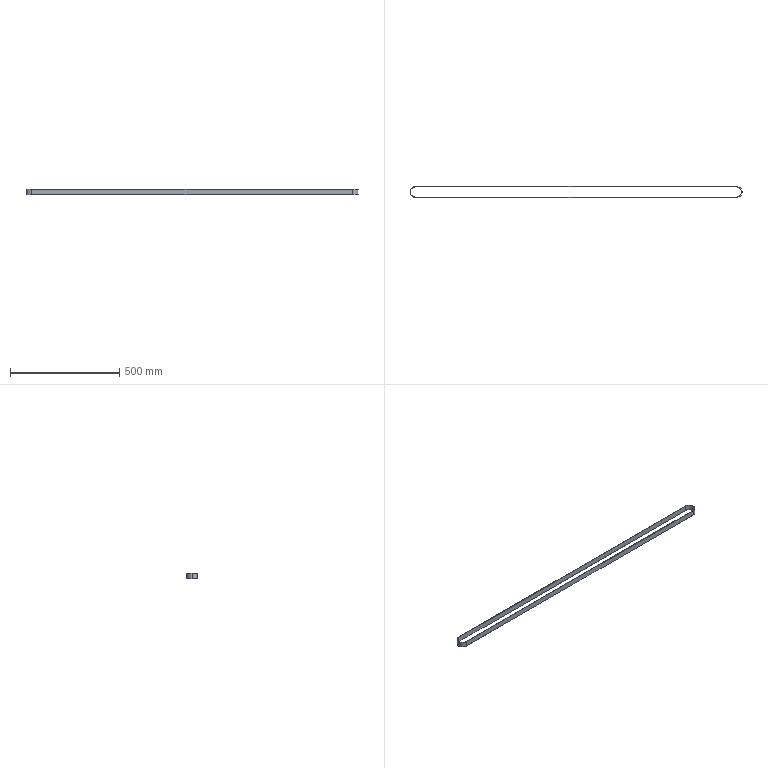Part | SolidWorks | features BaseBody 1 | 1 solid | 12 faces | box 1519 x 50.79 x 25 mm | volume 154464 mm3 | plane 6 | cylinder 6 | commonest cylinder face diameters 46.79 x3 50.79 x3
STEP:
#1=CARTESIAN_POINT('',(1368.,13.395,-12.5));
#2=VERTEX_POINT('',#1);
#3=CARTESIAN_POINT('',(-100.,13.395,-12.5));
#4=VERTEX_POINT('',#3);
#5=CARTESIAN_POINT('',(-100.,13.395,-12.5));
#6=DIRECTION('',(-1.,0.,0.));
#7=VECTOR('',#6,1000.);
#8=LINE('',#5,#7);
#9=EDGE_CURVE('',#2,#4,#8,.T.);
#10=ORIENTED_EDGE('',*,*,#9,.F.);
#11=CARTESIAN_POINT('',(1368.,13.395,12.5));
#12=VERTEX_POINT('',#11);
#13=CARTESIAN_POINT('',(1368.,13.395,12.5));
#14=DIRECTION('',(0.,0.,-1.));
#15=VECTOR('',#14,1000.);
#16=LINE('',#13,#15);
#17=EDGE_CURVE('',#12,#2,#16,.T.);
#18=ORIENTED_EDGE('',*,*,#17,.F.);
#19=CARTESIAN_POINT('',(-100.,13.395,12.5));
#20=VERTEX_POINT('',#19);
#21=CARTESIAN_POINT('',(-100.,13.395,12.5));
#22=DIRECTION('',(-1.,0.,0.));
#23=VECTOR('',#22,1000.);
#24=LINE('',#21,#23);
#25=EDGE_CURVE('',#12,#20,#24,.T.);
#26=ORIENTED_EDGE('',*,*,#25,.T.);
#27=CARTESIAN_POINT('',(-100.,13.395,12.5));
#28=DIRECTION('',(0.,0.,-1.));
#29=VECTOR('',#28,1000.);
#30=LINE('',#27,#29);
#31=EDGE_CURVE('',#20,#4,#30,.T.);
#32=ORIENTED_EDGE('',*,*,#31,.T.);
#33=EDGE_LOOP('',(#10,#18,#26,#32));
#34=FACE_OUTER_BOUND('',#33,.T.);
#35=CARTESIAN_POINT('',(-100.,13.395,12.5));
#36=DIRECTION('',(0.,-1.,0.));
#37=DIRECTION('',(0.,0.,-1.));
#38=AXIS2_PLACEMENT_3D('',#35,#36,#37);
#39=PLANE('',#38);
#40=ADVANCED_FACE('',(#34),#39,.T.);
#41=CARTESIAN_POINT('',(1368.,-33.395,-12.5));
#42=VERTEX_POINT('',#41);
#43=CARTESIAN_POINT('',(1368.,-10.,-12.5));
#44=DIRECTION('',(0.,0.,1.));
#45=DIRECTION('',(-1.,0.,0.));
#46=AXIS2_PLACEMENT_3D('',#43,#44,#45);
#47=CIRCLE('',#46,23.395);
#48=EDGE_CURVE('',#42,#2,#47,.T.);
#49=ORIENTED_EDGE('',*,*,#48,.F.);
#50=CARTESIAN_POINT('',(1368.,-33.395,12.5));
#51=VERTEX_POINT('',#50);
#52=CARTESIAN_POINT('',(1368.,-33.395,12.5));
#53=DIRECTION('',(0.,0.,-1.));
#54=VECTOR('',#53,1000.);
#55=LINE('',#52,#54);
#56=EDGE_CURVE('',#51,#42,#55,.T.);
#57=ORIENTED_EDGE('',*,*,#56,.F.);
#58=CARTESIAN_POINT('',(1368.,-10.,12.5));
#59=DIRECTION('',(0.,0.,1.));
#60=DIRECTION('',(-1.,0.,0.));
#61=AXIS2_PLACEMENT_3D('',#58,#59,#60);
#62=CIRCLE('',#61,23.395);
#63=EDGE_CURVE('',#51,#12,#62,.T.);
#64=ORIENTED_EDGE('',*,*,#63,.T.);
#65=ORIENTED_EDGE('',*,*,#17,.T.);
#66=EDGE_LOOP('',(#49,#57,#64,#65));
#67=FACE_OUTER_BOUND('',#66,.T.);
#68=CARTESIAN_POINT('',(1368.,-10.,12.5));
#69=DIRECTION('',(0.,0.,-1.));
#70=DIRECTION('',(-1.,0.,0.));
#71=AXIS2_PLACEMENT_3D('',#68,#69,#70);
#72=CYLINDRICAL_SURFACE('',#71,23.395);
#73=ADVANCED_FACE('',(#67),#72,.F.);
#74=CARTESIAN_POINT('',(-100.,-33.395,-12.5));
#75=VERTEX_POINT('',#74);
#76=CARTESIAN_POINT('',(1368.,-33.395,-12.5));
#77=DIRECTION('',(1.,0.,0.));
#78=VECTOR('',#77,1000.);
#79=LINE('',#76,#78);
#80=EDGE_CURVE('',#75,#42,#79,.T.);
#81=ORIENTED_EDGE('',*,*,#80,.F.);
#82=CARTESIAN_POINT('',(-100.,-33.395,12.5));
#83=VERTEX_POINT('',#82);
#84=CARTESIAN_POINT('',(-100.,-33.395,12.5));
#85=DIRECTION('',(0.,0.,-1.));
#86=VECTOR('',#85,1000.);
#87=LINE('',#84,#86);
#88=EDGE_CURVE('',#83,#75,#87,.T.);
#89=ORIENTED_EDGE('',*,*,#88,.F.);
#90=CARTESIAN_POINT('',(1368.,-33.395,12.5));
#91=DIRECTION('',(1.,0.,0.));
#92=VECTOR('',#91,1000.);
#93=LINE('',#90,#92);
#94=EDGE_CURVE('',#83,#51,#93,.T.);
#95=ORIENTED_EDGE('',*,*,#94,.T.);
#96=ORIENTED_EDGE('',*,*,#56,.T.);
#97=EDGE_LOOP('',(#81,#89,#95,#96));
#98=FACE_OUTER_BOUND('',#97,.T.);
#99=CARTESIAN_POINT('',(1368.,-33.395,12.5));
#100=DIRECTION('',(0.,1.,0.));
#101=DIRECTION('',(1.,0.,0.));
#102=AXIS2_PLACEMENT_3D('',#99,#100,#101);
#103=PLANE('',#102);
#104=ADVANCED_FACE('',(#98),#103,.T.);
#105=CARTESIAN_POINT('',(-123.395,-10.,12.5));
#106=VERTEX_POINT('',#105);
#107=CARTESIAN_POINT('',(-123.395,-10.,-12.5));
#108=VERTEX_POINT('',#107);
#109=CARTESIAN_POINT('',(-123.395,-10.,12.5));
#110=DIRECTION('',(0.,0.,-1.));
#111=VECTOR('',#110,1000.);
#112=LINE('',#109,#111);
#113=EDGE_CURVE('',#106,#108,#112,.T.);
#114=ORIENTED_EDGE('',*,*,#113,.F.);
#115=CARTESIAN_POINT('',(-100.,-10.,12.5));
#116=DIRECTION('',(0.,0.,1.));
#117=DIRECTION('',(-1.,0.,0.));
#118=AXIS2_PLACEMENT_3D('',#115,#116,#117);
#119=CIRCLE('',#118,23.395);
#120=EDGE_CURVE('',#106,#83,#119,.T.);
#121=ORIENTED_EDGE('',*,*,#120,.T.);
#122=ORIENTED_EDGE('',*,*,#88,.T.);
#123=CARTESIAN_POINT('',(-100.,-10.,-12.5));
#124=DIRECTION('',(0.,0.,1.));
#125=DIRECTION('',(-1.,0.,0.));
#126=AXIS2_PLACEMENT_3D('',#123,#124,#125);
#127=CIRCLE('',#126,23.395);
#128=EDGE_CURVE('',#108,#75,#127,.T.);
#129=ORIENTED_EDGE('',*,*,#128,.F.);
#130=EDGE_LOOP('',(#114,#121,#122,#129));
#131=FACE_OUTER_BOUND('',#130,.T.);
#132=CARTESIAN_POINT('',(-100.,-10.,12.5));
#133=DIRECTION('',(0.,0.,-1.));
#134=DIRECTION('',(-1.,0.,0.));
#135=AXIS2_PLACEMENT_3D('',#132,#133,#134);
#136=CYLINDRICAL_SURFACE('',#135,23.395);
#137=ADVANCED_FACE('',(#131),#136,.F.);
#138=CARTESIAN_POINT('',(1368.,15.395,-12.5));
#139=VERTEX_POINT('',#138);
#140=CARTESIAN_POINT('',(-100.,15.395,-12.5));
#141=VERTEX_POINT('',#140);
#142=CARTESIAN_POINT('',(-100.,15.395,-12.5));
#143=DIRECTION('',(-1.,0.,0.));
#144=VECTOR('',#143,1000.);
#145=LINE('',#142,#144);
#146=EDGE_CURVE('',#139,#141,#145,.T.);
#147=ORIENTED_EDGE('',*,*,#146,.T.);
#148=CARTESIAN_POINT('',(-100.,15.395,12.5));
#149=VERTEX_POINT('',#148);
#150=CARTESIAN_POINT('',(-100.,15.395,12.5));
#151=DIRECTION('',(0.,0.,-1.));
#152=VECTOR('',#151,1000.);
#153=LINE('',#150,#152);
#154=EDGE_CURVE('',#149,#141,#153,.T.);
#155=ORIENTED_EDGE('',*,*,#154,.F.);
#156=CARTESIAN_POINT('',(1368.,15.395,12.5));
#157=VERTEX_POINT('',#156);
#158=CARTESIAN_POINT('',(-100.,15.395,12.5));
#159=DIRECTION('',(-1.,0.,0.));
#160=VECTOR('',#159,1000.);
#161=LINE('',#158,#160);
#162=EDGE_CURVE('',#157,#149,#161,.T.);
#163=ORIENTED_EDGE('',*,*,#162,.F.);
#164=CARTESIAN_POINT('',(1368.,15.395,12.5));
#165=DIRECTION('',(0.,0.,-1.));
#166=VECTOR('',#165,1000.);
#167=LINE('',#164,#166);
#168=EDGE_CURVE('',#157,#139,#167,.T.);
#169=ORIENTED_EDGE('',*,*,#168,.T.);
#170=EDGE_LOOP('',(#147,#155,#163,#169));
#171=FACE_OUTER_BOUND('',#170,.T.);
#172=CARTESIAN_POINT('',(-100.,15.395,12.5));
#173=DIRECTION('',(0.,-1.,0.));
#174=DIRECTION('',(0.,0.,-1.));
#175=AXIS2_PLACEMENT_3D('',#172,#173,#174);
#176=PLANE('',#175);
#177=ADVANCED_FACE('',(#171),#176,.F.);
#178=CARTESIAN_POINT('',(1368.,-35.395,-12.5));
#179=VERTEX_POINT('',#178);
#180=CARTESIAN_POINT('',(1368.,-10.,-12.5));
#181=DIRECTION('',(0.,0.,1.));
#182=DIRECTION('',(-1.,0.,0.));
#183=AXIS2_PLACEMENT_3D('',#180,#181,#182);
#184=CIRCLE('',#183,25.395);
#185=EDGE_CURVE('',#179,#139,#184,.T.);
#186=ORIENTED_EDGE('',*,*,#185,.T.);
#187=ORIENTED_EDGE('',*,*,#168,.F.);
#188=CARTESIAN_POINT('',(1368.,-35.395,12.5));
#189=VERTEX_POINT('',#188);
#190=CARTESIAN_POINT('',(1368.,-10.,12.5));
#191=DIRECTION('',(0.,0.,1.));
#192=DIRECTION('',(-1.,0.,0.));
#193=AXIS2_PLACEMENT_3D('',#190,#191,#192);
#194=CIRCLE('',#193,25.395);
#195=EDGE_CURVE('',#189,#157,#194,.T.);
#196=ORIENTED_EDGE('',*,*,#195,.F.);
#197=CARTESIAN_POINT('',(1368.,-35.395,12.5));
#198=DIRECTION('',(0.,0.,-1.));
#199=VECTOR('',#198,1000.);
#200=LINE('',#197,#199);
#201=EDGE_CURVE('',#189,#179,#200,.T.);
#202=ORIENTED_EDGE('',*,*,#201,.T.);
#203=EDGE_LOOP('',(#186,#187,#196,#202));
#204=FACE_OUTER_BOUND('',#203,.T.);
#205=CARTESIAN_POINT('',(1368.,-10.,12.5));
#206=DIRECTION('',(0.,0.,-1.));
#207=DIRECTION('',(-1.,0.,0.));
#208=AXIS2_PLACEMENT_3D('',#205,#206,#207);
#209=CYLINDRICAL_SURFACE('',#208,25.395);
#210=ADVANCED_FACE('',(#204),#209,.T.);
#211=CARTESIAN_POINT('',(-100.,-35.395,-12.5));
#212=VERTEX_POINT('',#211);
#213=CARTESIAN_POINT('',(-100.,-35.395,-12.5));
#214=DIRECTION('',(1.,0.,0.));
#215=VECTOR('',#214,1000.);
#216=LINE('',#213,#215);
#217=EDGE_CURVE('',#212,#179,#216,.T.);
#218=ORIENTED_EDGE('',*,*,#217,.T.);
#219=ORIENTED_EDGE('',*,*,#201,.F.);
#220=CARTESIAN_POINT('',(-100.,-35.395,12.5));
#221=VERTEX_POINT('',#220);
#222=CARTESIAN_POINT('',(-100.,-35.395,12.5));
#223=DIRECTION('',(1.,0.,0.));
#224=VECTOR('',#223,1000.);
#225=LINE('',#222,#224);
#226=EDGE_CURVE('',#221,#189,#225,.T.);
#227=ORIENTED_EDGE('',*,*,#226,.F.);
#228=CARTESIAN_POINT('',(-100.,-35.395,12.5));
#229=DIRECTION('',(0.,0.,-1.));
#230=VECTOR('',#229,1000.);
#231=LINE('',#228,#230);
#232=EDGE_CURVE('',#221,#212,#231,.T.);
#233=ORIENTED_EDGE('',*,*,#232,.T.);
#234=EDGE_LOOP('',(#218,#219,#227,#233));
#235=FACE_OUTER_BOUND('',#234,.T.);
#236=CARTESIAN_POINT('',(-100.,-35.395,12.5));
#237=DIRECTION('',(0.,1.,0.));
#238=DIRECTION('',(1.,0.,0.));
#239=AXIS2_PLACEMENT_3D('',#236,#237,#238);
#240=PLANE('',#239);
#241=ADVANCED_FACE('',(#235),#240,.F.);
#242=CARTESIAN_POINT('',(-125.395,-10.,12.5));
#243=VERTEX_POINT('',#242);
#244=CARTESIAN_POINT('',(-125.395,-10.,-12.5));
#245=VERTEX_POINT('',#244);
#246=CARTESIAN_POINT('',(-125.395,-10.,12.5));
#247=DIRECTION('',(0.,0.,-1.));
#248=VECTOR('',#247,1000.);
#249=LINE('',#246,#248);
#250=EDGE_CURVE('',#243,#245,#249,.T.);
#251=ORIENTED_EDGE('',*,*,#250,.F.);
#252=CARTESIAN_POINT('',(-100.,-10.,12.5));
#253=DIRECTION('',(0.,0.,1.));
#254=DIRECTION('',(-1.,0.,0.));
#255=AXIS2_PLACEMENT_3D('',#252,#253,#254);
#256=CIRCLE('',#255,25.395);
#257=EDGE_CURVE('',#149,#243,#256,.T.);
#258=ORIENTED_EDGE('',*,*,#257,.F.);
#259=ORIENTED_EDGE('',*,*,#154,.T.);
#260=CARTESIAN_POINT('',(-100.,-10.,-12.5));
#261=DIRECTION('',(0.,0.,1.));
#262=DIRECTION('',(-1.,0.,0.));
#263=AXIS2_PLACEMENT_3D('',#260,#261,#262);
#264=CIRCLE('',#263,25.395);
#265=EDGE_CURVE('',#141,#245,#264,.T.);
#266=ORIENTED_EDGE('',*,*,#265,.T.);
#267=EDGE_LOOP('',(#251,#258,#259,#266));
#268=FACE_OUTER_BOUND('',#267,.T.);
#269=CARTESIAN_POINT('',(-100.,-10.,12.5));
#270=DIRECTION('',(0.,0.,-1.));
#271=DIRECTION('',(-1.,0.,0.));
#272=AXIS2_PLACEMENT_3D('',#269,#270,#271);
#273=CYLINDRICAL_SURFACE('',#272,25.395);
#274=ADVANCED_FACE('',(#268),#273,.T.);
#275=ORIENTED_EDGE('',*,*,#9,.T.);
#276=CARTESIAN_POINT('',(-100.,-10.,-12.5));
#277=DIRECTION('',(0.,0.,1.));
#278=DIRECTION('',(-1.,0.,0.));
#279=AXIS2_PLACEMENT_3D('',#276,#277,#278);
#280=CIRCLE('',#279,23.395);
#281=EDGE_CURVE('',#4,#108,#280,.T.);
#282=ORIENTED_EDGE('',*,*,#281,.T.);
#283=ORIENTED_EDGE('',*,*,#128,.T.);
#284=ORIENTED_EDGE('',*,*,#80,.T.);
#285=ORIENTED_EDGE('',*,*,#48,.T.);
#286=EDGE_LOOP('',(#275,#282,#283,#284,#285));
#287=FACE_BOUND('',#286,.T.);
#288=ORIENTED_EDGE('',*,*,#265,.F.);
#289=ORIENTED_EDGE('',*,*,#146,.F.);
#290=ORIENTED_EDGE('',*,*,#185,.F.);
#291=ORIENTED_EDGE('',*,*,#217,.F.);
#292=CARTESIAN_POINT('',(-100.,-10.,-12.5));
#293=DIRECTION('',(0.,0.,1.));
#294=DIRECTION('',(-1.,0.,0.));
#295=AXIS2_PLACEMENT_3D('',#292,#293,#294);
#296=CIRCLE('',#295,25.395);
#297=EDGE_CURVE('',#245,#212,#296,.T.);
#298=ORIENTED_EDGE('',*,*,#297,.F.);
#299=EDGE_LOOP('',(#288,#289,#290,#291,#298));
#300=FACE_OUTER_BOUND('',#299,.T.);
#301=CARTESIAN_POINT('',(-100.,-10.,-12.5));
#302=DIRECTION('',(0.,0.,-1.));
#303=DIRECTION('',(0.,-1.,0.));
#304=AXIS2_PLACEMENT_3D('',#301,#302,#303);
#305=PLANE('',#304);
#306=ADVANCED_FACE('',(#287,#300),#305,.T.);
#307=CARTESIAN_POINT('',(-100.,-10.,12.5));
#308=DIRECTION('',(0.,0.,1.));
#309=DIRECTION('',(-1.,0.,0.));
#310=AXIS2_PLACEMENT_3D('',#307,#308,#309);
#311=CIRCLE('',#310,23.395);
#312=EDGE_CURVE('',#20,#106,#311,.T.);
#313=ORIENTED_EDGE('',*,*,#312,.F.);
#314=ORIENTED_EDGE('',*,*,#25,.F.);
#315=ORIENTED_EDGE('',*,*,#63,.F.);
#316=ORIENTED_EDGE('',*,*,#94,.F.);
#317=ORIENTED_EDGE('',*,*,#120,.F.);
#318=EDGE_LOOP('',(#313,#314,#315,#316,#317));
#319=FACE_BOUND('',#318,.T.);
#320=ORIENTED_EDGE('',*,*,#257,.T.);
#321=CARTESIAN_POINT('',(-100.,-10.,12.5));
#322=DIRECTION('',(0.,0.,1.));
#323=DIRECTION('',(-1.,0.,0.));
#324=AXIS2_PLACEMENT_3D('',#321,#322,#323);
#325=CIRCLE('',#324,25.395);
#326=EDGE_CURVE('',#243,#221,#325,.T.);
#327=ORIENTED_EDGE('',*,*,#326,.T.);
#328=ORIENTED_EDGE('',*,*,#226,.T.);
#329=ORIENTED_EDGE('',*,*,#195,.T.);
#330=ORIENTED_EDGE('',*,*,#162,.T.);
#331=EDGE_LOOP('',(#320,#327,#328,#329,#330));
#332=FACE_OUTER_BOUND('',#331,.T.);
#333=CARTESIAN_POINT('',(-100.,-10.,12.5));
#334=DIRECTION('',(0.,0.,-1.));
#335=DIRECTION('',(0.,-1.,0.));
#336=AXIS2_PLACEMENT_3D('',#333,#334,#335);
#337=PLANE('',#336);
#338=ADVANCED_FACE('',(#319,#332),#337,.F.);
#339=ORIENTED_EDGE('',*,*,#326,.F.);
#340=ORIENTED_EDGE('',*,*,#250,.T.);
#341=ORIENTED_EDGE('',*,*,#297,.T.);
#342=ORIENTED_EDGE('',*,*,#232,.F.);
#343=EDGE_LOOP('',(#339,#340,#341,#342));
#344=FACE_OUTER_BOUND('',#343,.T.);
#345=CARTESIAN_POINT('',(-100.,-10.,12.5));
#346=DIRECTION('',(0.,0.,-1.));
#347=DIRECTION('',(-1.,0.,0.));
#348=AXIS2_PLACEMENT_3D('',#345,#346,#347);
#349=CYLINDRICAL_SURFACE('',#348,25.395);
#350=ADVANCED_FACE('',(#344),#349,.T.);
#351=ORIENTED_EDGE('',*,*,#312,.T.);
#352=ORIENTED_EDGE('',*,*,#113,.T.);
#353=ORIENTED_EDGE('',*,*,#281,.F.);
#354=ORIENTED_EDGE('',*,*,#31,.F.);
#355=EDGE_LOOP('',(#351,#352,#353,#354));
#356=FACE_OUTER_BOUND('',#355,.T.);
#357=CARTESIAN_POINT('',(-100.,-10.,12.5));
#358=DIRECTION('',(0.,0.,-1.));
#359=DIRECTION('',(-1.,0.,0.));
#360=AXIS2_PLACEMENT_3D('',#357,#358,#359);
#361=CYLINDRICAL_SURFACE('',#360,23.395);
#362=ADVANCED_FACE('',(#356),#361,.F.);
#363=CLOSED_SHELL('',(#40,#73,#104,#137,#177,#210,#241,#274,#306,#338,#350,#362));
#364=MANIFOLD_SOLID_BREP('',#363);
#365=CARTESIAN_POINT('',(0.,0.,0.));
#366=DIRECTION('',(0.,0.,1.));
#367=DIRECTION('',(1.,0.,0.));
#368=AXIS2_PLACEMENT_3D('',#365,#366,#367);
#369=(LENGTH_UNIT()NAMED_UNIT(*)SI_UNIT(.MILLI.,.METRE.));
#370=UNCERTAINTY_MEASURE_WITH_UNIT(LENGTH_MEASURE(0.00001),#369,'','');
#371=(NAMED_UNIT(*)PLANE_ANGLE_UNIT()SI_UNIT($,.RADIAN.));
#372=(NAMED_UNIT(*)SI_UNIT($,.STERADIAN.)SOLID_ANGLE_UNIT());
#373=(GEOMETRIC_REPRESENTATION_CONTEXT(3)GLOBAL_UNCERTAINTY_ASSIGNED_CONTEXT((#370))GLOBAL_UNIT_ASSIGNED_CONTEXT((#369,#371,#372))REPRESENTATION_CONTEXT('',''));
#374=ADVANCED_BREP_SHAPE_REPRESENTATION('',(#364,#368),#373);